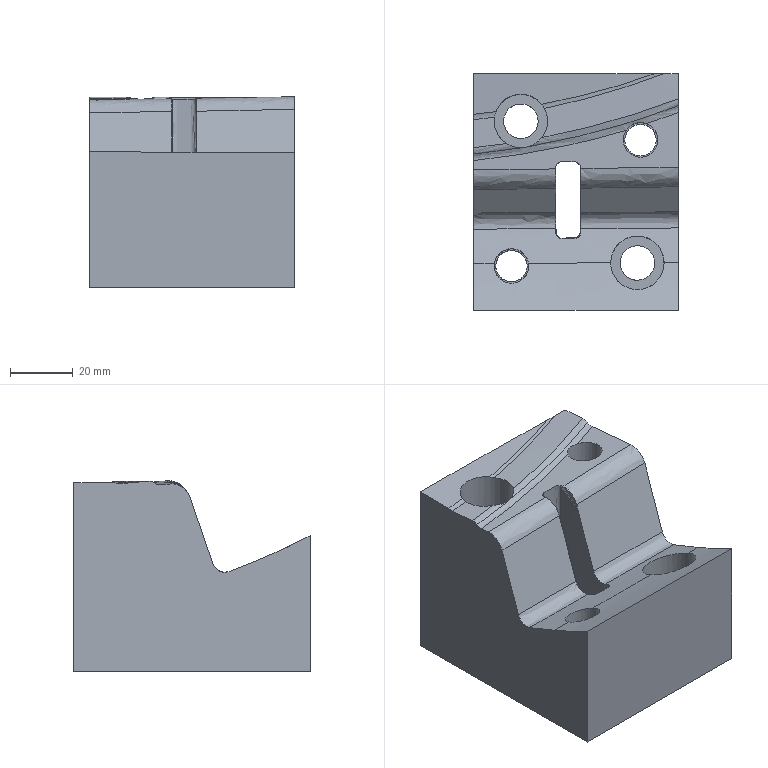Part | NX | features solid 2 | 1 solid | 46 faces | box 65.001 x 75 x 60.535 mm | volume 200361 mm3 | spline 29 | plane 9 | cylinder 8 | commonest cylinder face diameters 11 x4 10 x2 17 x2